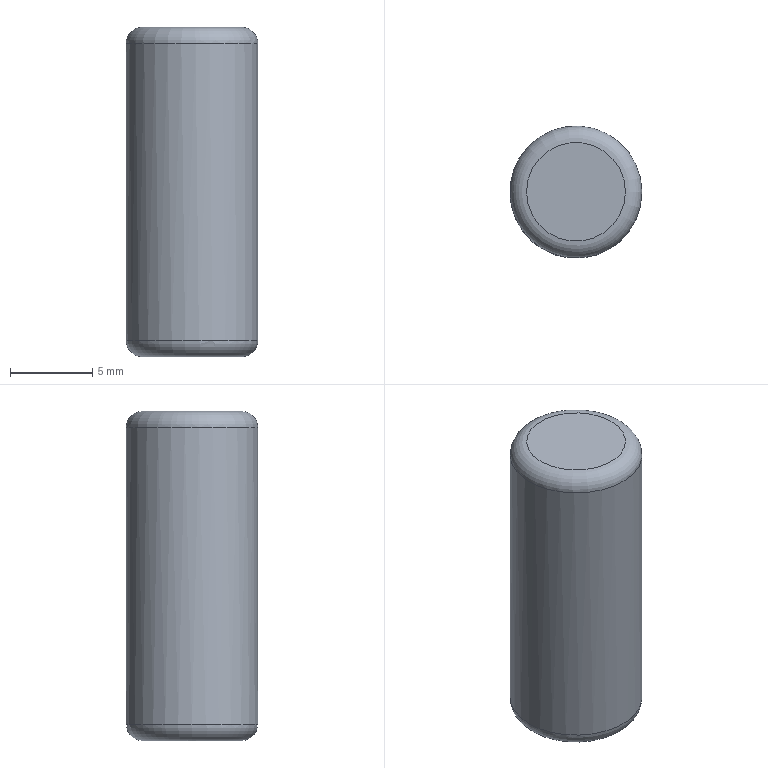Part | STEP file | 200 mesh_id714_x | 1 solid | 5 faces | box 8 x 8 x 20 mm | volume 995.125 mm3 | plane 2 | torus 2 | cylinder 1 | commonest cylinder face diameters 8 x1
STEP:
#1=CARTESIAN_POINT('',(-16794.884,-4110.269,10.));
#2=VERTEX_POINT('',#1);
#3=CARTESIAN_POINT('',(-16797.884,-4110.269,10.));
#4=DIRECTION('',(0.,0.,1.));
#5=DIRECTION('',(1.,0.,0.));
#6=AXIS2_PLACEMENT_3D('',#3,#4,#5);
#7=CIRCLE('',#6,3.);
#8=EDGE_CURVE('',#2,#2,#7,.T.);
#9=ORIENTED_EDGE('',*,*,#8,.T.);
#10=EDGE_LOOP('',(#9));
#11=FACE_OUTER_BOUND('',#10,.T.);
#12=CARTESIAN_POINT('',(-16797.884,-4110.269,10.));
#13=DIRECTION('',(0.,0.,1.));
#14=DIRECTION('',(1.,0.,0.));
#15=AXIS2_PLACEMENT_3D('',#12,#13,#14);
#16=PLANE('',#15);
#17=ADVANCED_FACE('',(#11),#16,.T.);
#18=CARTESIAN_POINT('',(-16800.884,-4110.269,-10.));
#19=VERTEX_POINT('',#18);
#20=CARTESIAN_POINT('',(-16797.884,-4110.269,-10.));
#21=DIRECTION('',(0.,0.,-1.));
#22=DIRECTION('',(-1.,0.,0.));
#23=AXIS2_PLACEMENT_3D('',#20,#21,#22);
#24=CIRCLE('',#23,3.);
#25=EDGE_CURVE('',#19,#19,#24,.T.);
#26=ORIENTED_EDGE('',*,*,#25,.T.);
#27=EDGE_LOOP('',(#26));
#28=FACE_OUTER_BOUND('',#27,.T.);
#29=CARTESIAN_POINT('',(-16797.884,-4110.269,-10.));
#30=DIRECTION('',(0.,0.,-1.));
#31=DIRECTION('',(-1.,0.,0.));
#32=AXIS2_PLACEMENT_3D('',#29,#30,#31);
#33=PLANE('',#32);
#34=ADVANCED_FACE('',(#28),#33,.T.);
#35=CARTESIAN_POINT('',(-16801.884,-4110.269,-9.));
#36=VERTEX_POINT('',#35);
#37=CARTESIAN_POINT('',(-16797.884,-4110.269,-9.));
#38=DIRECTION('',(0.,0.,1.));
#39=DIRECTION('',(-1.,0.,0.));
#40=AXIS2_PLACEMENT_3D('',#37,#38,#39);
#41=CIRCLE('',#40,4.);
#42=EDGE_CURVE('',#36,#36,#41,.T.);
#43=ORIENTED_EDGE('',*,*,#42,.T.);
#44=EDGE_LOOP('',(#43));
#45=FACE_BOUND('',#44,.T.);
#46=CARTESIAN_POINT('',(-16793.884,-4110.269,9.));
#47=VERTEX_POINT('',#46);
#48=CARTESIAN_POINT('',(-16797.884,-4110.269,9.));
#49=DIRECTION('',(0.,0.,-1.));
#50=DIRECTION('',(1.,0.,0.));
#51=AXIS2_PLACEMENT_3D('',#48,#49,#50);
#52=CIRCLE('',#51,4.);
#53=EDGE_CURVE('',#47,#47,#52,.T.);
#54=ORIENTED_EDGE('',*,*,#53,.T.);
#55=EDGE_LOOP('',(#54));
#56=FACE_BOUND('',#55,.T.);
#57=CARTESIAN_POINT('',(-16797.884,-4110.269,0.));
#58=DIRECTION('',(0.,0.,1.));
#59=DIRECTION('',(1.,0.,0.));
#60=AXIS2_PLACEMENT_3D('',#57,#58,#59);
#61=CYLINDRICAL_SURFACE('',#60,4.);
#62=ADVANCED_FACE('',(#45,#56),#61,.T.);
#63=ORIENTED_EDGE('',*,*,#25,.F.);
#64=EDGE_LOOP('',(#63));
#65=FACE_BOUND('',#64,.T.);
#66=ORIENTED_EDGE('',*,*,#42,.F.);
#67=EDGE_LOOP('',(#66));
#68=FACE_BOUND('',#67,.T.);
#69=CARTESIAN_POINT('',(-16797.884,-4110.269,-9.));
#70=DIRECTION('',(0.,0.,-1.));
#71=DIRECTION('',(-1.,0.,0.));
#72=AXIS2_PLACEMENT_3D('',#69,#70,#71);
#73=TOROIDAL_SURFACE('',#72,3.,1.);
#74=ADVANCED_FACE('',(#65,#68),#73,.T.);
#75=ORIENTED_EDGE('',*,*,#8,.F.);
#76=EDGE_LOOP('',(#75));
#77=FACE_BOUND('',#76,.T.);
#78=ORIENTED_EDGE('',*,*,#53,.F.);
#79=EDGE_LOOP('',(#78));
#80=FACE_BOUND('',#79,.T.);
#81=CARTESIAN_POINT('',(-16797.884,-4110.269,9.));
#82=DIRECTION('',(0.,0.,1.));
#83=DIRECTION('',(1.,0.,0.));
#84=AXIS2_PLACEMENT_3D('',#81,#82,#83);
#85=TOROIDAL_SURFACE('',#84,3.,1.);
#86=ADVANCED_FACE('',(#77,#80),#85,.T.);
#87=CLOSED_SHELL('',(#17,#34,#62,#74,#86));
#88=MANIFOLD_SOLID_BREP('',#87);
#89=(LENGTH_UNIT()NAMED_UNIT(*)SI_UNIT(.MILLI.,.METRE.));
#90=UNCERTAINTY_MEASURE_WITH_UNIT(LENGTH_MEASURE(0.00002),#89,'','');
#91=(NAMED_UNIT(*)PLANE_ANGLE_UNIT()SI_UNIT($,.RADIAN.));
#92=PLANE_ANGLE_MEASURE_WITH_UNIT(PLANE_ANGLE_MEASURE(0.01745),#91);
#93=DIMENSIONAL_EXPONENTS(0.,0.,0.,0.,0.,0.,0.);
#94=(CONVERSION_BASED_UNIT('DEGREE',#92)NAMED_UNIT(#93)PLANE_ANGLE_UNIT());
#95=(NAMED_UNIT(*)SI_UNIT($,.STERADIAN.)SOLID_ANGLE_UNIT());
#96=(GEOMETRIC_REPRESENTATION_CONTEXT(3)GLOBAL_UNCERTAINTY_ASSIGNED_CONTEXT((#90))GLOBAL_UNIT_ASSIGNED_CONTEXT((#89,#94,#95))REPRESENTATION_CONTEXT('',''));
#97=ADVANCED_BREP_SHAPE_REPRESENTATION('',(#88),#96);